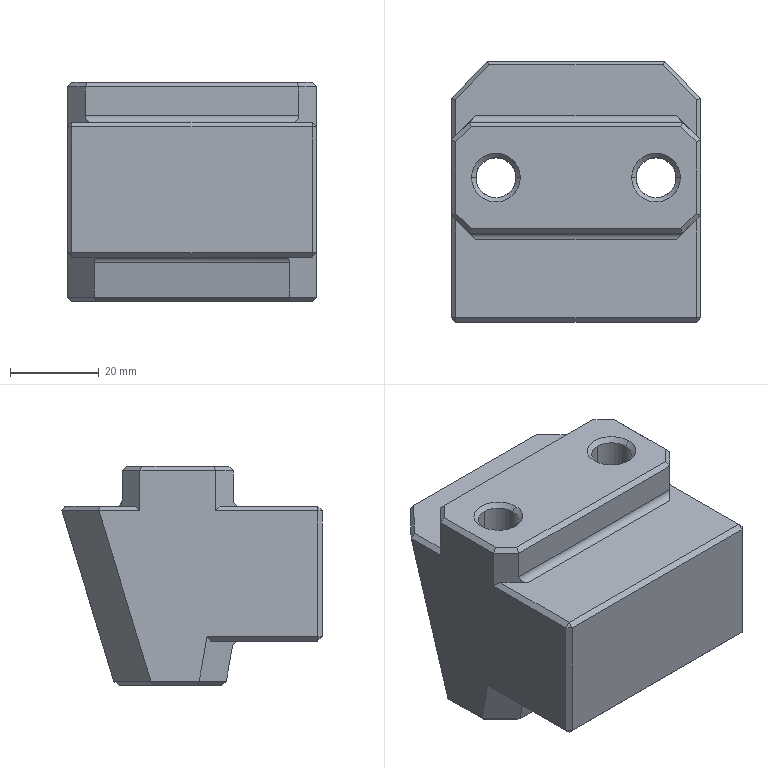Part | Creo | 1 solid | 74 faces | box 56 x 58.606 x 49.267 mm | volume 108262 mm3 | plane 55 | cylinder 11 | cone 8 | commonest cylinder face diameters 9 x4 14 x4 3 x3